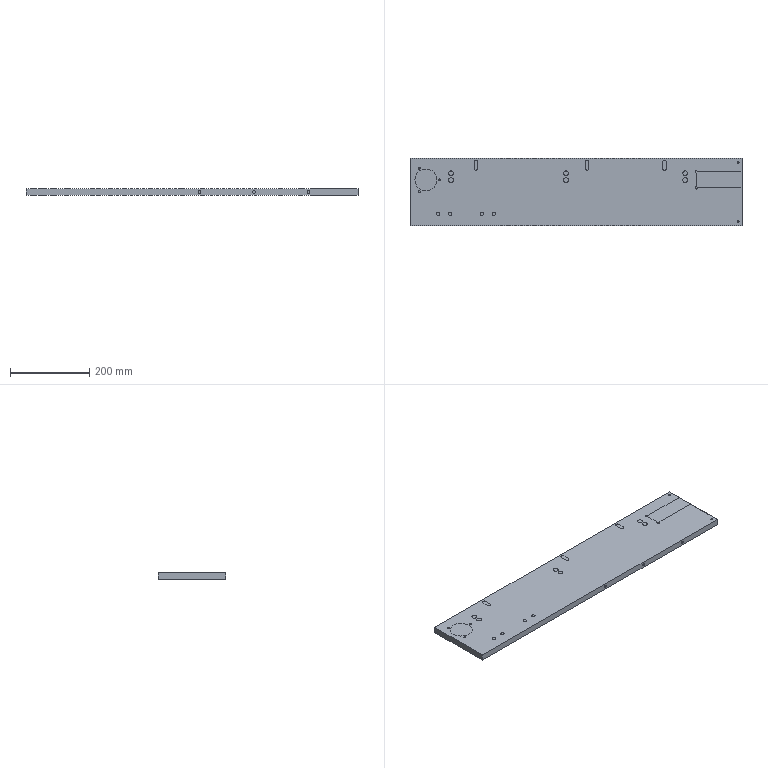NC program | NX | posted with a generic post | part box 836 x 170 x 16 mm
Lines 238 to 1148 of 11551:
(等高外形_2 , TOOL : D8平底刀)
N462 T15 M6
N464 /M1
N466 G17 G43 G0 G90 X640.643 Y150.661 Z100. S2600 H15 M3
N468 Z0.
N470 G94 G1 Z-0.2 F1200.
N472 G3 X641.5 Y152.5 R2.4
N474 G1 Y160.5 F1500.
N476 G3 X641. Y161. R0.5
N478 X640.5 Y160.5 R0.5
N480 G1 Y144.5
N482 G3 X641. Y144. R0.5
N484 X641.5 Y144.5 R0.5
N486 G1 Y152.5
N488 Y160.5 Z-0.246
N490 X641.483 Y160.628
N492 X641.463 Y160.689 Z-0.247
N494 X641.407 Y160.79
N496 X641.357 Y160.85 Z-0.248
N498 X641.269 Y160.922
N500 X641.199 Y160.959 Z-0.249
N502 X641.088 Y160.992 Z-0.25
N504 X641.006 Y161.
N506 X640.891 Y160.988 Z-0.251
N508 X640.813 Y160.964
N510 X640.712 Y160.909 Z-0.252
N512 X640.649 Y160.856
N514 X640.576 Y160.766 Z-0.253
N516 X640.539 Y160.693
N518 X640.513 Y160.615 Z-0.254
N520 X640.5 Y160.5
N522 Y144.5 Z-0.346
N524 X640.517 Y144.37
N526 X640.539 Y144.307 Z-0.347
N528 X640.597 Y144.204
N530 X640.649 Y144.144 Z-0.348
N532 X640.74 Y144.073
N534 X640.814 Y144.036 Z-0.349
N536 X640.925 Y144.006 Z-0.35
N538 X641.007 Y144.
N540 X641.121 Y144.015 Z-0.351
N542 X641.199 Y144.041
N544 X641.297 Y144.098 Z-0.352
N546 X641.358 Y144.151
N548 X641.427 Y144.24 Z-0.353
N550 X641.463 Y144.311
N552 X641.487 Y144.388 Z-0.354
N554 X641.5 Y144.5
N556 Y152.5 Z-0.4
N558 Y160.5 Z-0.446
N560 X641.483 Y160.628
N562 X641.463 Y160.689 Z-0.447
N564 X641.407 Y160.79
N566 X641.357 Y160.85 Z-0.448
N568 X641.269 Y160.922
N570 X641.199 Y160.959 Z-0.449
N572 X641.088 Y160.992 Z-0.45
N574 X641.006 Y161.
N576 X640.891 Y160.988 Z-0.451
N578 X640.813 Y160.964
N580 X640.712 Y160.909 Z-0.452
N582 X640.649 Y160.856
N584 X640.576 Y160.766 Z-0.453
N586 X640.539 Y160.693
N588 X640.513 Y160.615 Z-0.454
N590 X640.5 Y160.5
N592 Y144.5 Z-0.546
N594 X640.517 Y144.37
N596 X640.539 Y144.307 Z-0.547
N598 X640.597 Y144.204
N600 X640.649 Y144.144 Z-0.548
N602 X640.74 Y144.073
N604 X640.814 Y144.036 Z-0.549
N606 X640.925 Y144.006 Z-0.55
N608 X641.007 Y144.
N610 X641.121 Y144.015 Z-0.551
N612 X641.199 Y144.041
N614 X641.297 Y144.098 Z-0.552
N616 X641.358 Y144.151
N618 X641.427 Y144.24 Z-0.553
N620 X641.463 Y144.311
N622 X641.487 Y144.388 Z-0.554
N624 X641.5 Y144.5
N626 Y152.5 Z-0.6
N628 Y160.5 Z-0.646
N630 X641.483 Y160.628
N632 X641.463 Y160.689 Z-0.647
N634 X641.407 Y160.79
N636 X641.357 Y160.85 Z-0.648
N638 X641.269 Y160.922
N640 X641.199 Y160.959 Z-0.649
N642 X641.088 Y160.992 Z-0.65
N644 X641.006 Y161.
N646 X640.891 Y160.988 Z-0.651
N648 X640.813 Y160.964
N650 X640.712 Y160.909 Z-0.652
N652 X640.649 Y160.856
N654 X640.576 Y160.766 Z-0.653
N656 X640.539 Y160.693
N658 X640.513 Y160.615 Z-0.654
N660 X640.5 Y160.5
N662 Y144.5 Z-0.746
N664 X640.517 Y144.37
N666 X640.539 Y144.307 Z-0.747
N668 X640.597 Y144.204
N670 X640.649 Y144.144 Z-0.748
N672 X640.74 Y144.073
N674 X640.814 Y144.036 Z-0.749
N676 X640.925 Y144.006 Z-0.75
N678 X641.007 Y144.
N680 X641.121 Y144.015 Z-0.751
N682 X641.199 Y144.041
N684 X641.297 Y144.098 Z-0.752
N686 X641.358 Y144.151
N688 X641.427 Y144.24 Z-0.753
N690 X641.463 Y144.311
N692 X641.487 Y144.388 Z-0.754
N694 X641.5 Y144.5
N696 Y152.5 Z-0.8
N698 Y160.5 Z-0.846
N700 X641.483 Y160.628
N702 X641.463 Y160.689 Z-0.847
N704 X641.407 Y160.79
N706 X641.357 Y160.85 Z-0.848
N708 X641.269 Y160.922
N710 X641.199 Y160.959 Z-0.849
N712 X641.088 Y160.992 Z-0.85
N714 X641.006 Y161.
N716 X640.891 Y160.988 Z-0.851
N718 X640.813 Y160.964
N720 X640.712 Y160.909 Z-0.852
N722 X640.649 Y160.856
N724 X640.576 Y160.766 Z-0.853
N726 X640.539 Y160.693
N728 X640.513 Y160.615 Z-0.854
N730 X640.5 Y160.5
N732 Y144.5 Z-0.946
N734 X640.517 Y144.37
N736 X640.539 Y144.307 Z-0.947
N738 X640.597 Y144.204
N740 X640.649 Y144.144 Z-0.948
N742 X640.74 Y144.073
N744 X640.814 Y144.036 Z-0.949
N746 X640.925 Y144.006 Z-0.95
N748 X641.007 Y144.
N750 X641.121 Y144.015 Z-0.951
N752 X641.199 Y144.041
N754 X641.297 Y144.098 Z-0.952
N756 X641.358 Y144.151
N758 X641.427 Y144.24 Z-0.953
N760 X641.463 Y144.311
N762 X641.487 Y144.388 Z-0.954
N764 X641.5 Y144.5
N766 Y152.5 Z-1.
N768 Y160.5 Z-1.046
N770 X641.483 Y160.628
N772 X641.463 Y160.689 Z-1.047
N774 X641.407 Y160.79
N776 X641.357 Y160.85 Z-1.048
N778 X641.269 Y160.922
N780 X641.199 Y160.959 Z-1.049
N782 X641.088 Y160.992 Z-1.05
N784 X641.006 Y161.
N786 X640.891 Y160.988 Z-1.051
N788 X640.813 Y160.964
N790 X640.712 Y160.909 Z-1.052
N792 X640.649 Y160.856
N794 X640.576 Y160.766 Z-1.053
N796 X640.539 Y160.693
N798 X640.513 Y160.615 Z-1.054
N800 X640.5 Y160.5
N802 Y144.5 Z-1.146
N804 X640.517 Y144.37
N806 X640.539 Y144.307 Z-1.147
N808 X640.597 Y144.204
N810 X640.649 Y144.144 Z-1.148
N812 X640.74 Y144.073
N814 X640.814 Y144.036 Z-1.149
N816 X640.925 Y144.006 Z-1.15
N818 X641.007 Y144.
N820 X641.121 Y144.015 Z-1.151
N822 X641.199 Y144.041
N824 X641.297 Y144.098 Z-1.152
N826 X641.358 Y144.151
N828 X641.427 Y144.24 Z-1.153
N830 X641.463 Y144.311
N832 X641.487 Y144.388 Z-1.154
N834 X641.5 Y144.5
N836 Y152.5 Z-1.2
N838 Y160.5 Z-1.246
N840 X641.483 Y160.628
N842 X641.463 Y160.689 Z-1.247
N844 X641.407 Y160.79
N846 X641.357 Y160.85 Z-1.248
N848 X641.269 Y160.922
N850 X641.199 Y160.959 Z-1.249
N852 X641.088 Y160.992 Z-1.25
N854 X641.006 Y161.
N856 X640.891 Y160.988 Z-1.251
N858 X640.813 Y160.964
N860 X640.712 Y160.909 Z-1.252
N862 X640.649 Y160.856
N864 X640.576 Y160.766 Z-1.253
N866 X640.539 Y160.693
N868 X640.513 Y160.615 Z-1.254
N870 X640.5 Y160.5
N872 Y144.5 Z-1.346
N874 X640.517 Y144.37
N876 X640.539 Y144.307 Z-1.347
N878 X640.597 Y144.204
N880 X640.649 Y144.144 Z-1.348
N882 X640.74 Y144.073
N884 X640.814 Y144.036 Z-1.349
N886 X640.925 Y144.006 Z-1.35
N888 X641.007 Y144.
N890 X641.121 Y144.015 Z-1.351
N892 X641.199 Y144.041
N894 X641.297 Y144.098 Z-1.352
N896 X641.358 Y144.151
N898 X641.427 Y144.24 Z-1.353
N900 X641.463 Y144.311
N902 X641.487 Y144.388 Z-1.354
N904 X641.5 Y144.5
N906 Y152.5 Z-1.4
N908 Y160.5 Z-1.446
N910 X641.483 Y160.628
N912 X641.463 Y160.689 Z-1.447
N914 X641.407 Y160.79
N916 X641.357 Y160.85 Z-1.448
N918 X641.269 Y160.922
N920 X641.199 Y160.959 Z-1.449
N922 X641.088 Y160.992 Z-1.45
N924 X641.006 Y161.
N926 X640.891 Y160.988 Z-1.451
N928 X640.813 Y160.964
N930 X640.712 Y160.909 Z-1.452
N932 X640.649 Y160.856
N934 X640.576 Y160.766 Z-1.453
N936 X640.539 Y160.693
N938 X640.513 Y160.615 Z-1.454
N940 X640.5 Y160.5
N942 Y144.5 Z-1.546
N944 X640.517 Y144.37
N946 X640.539 Y144.307 Z-1.547
N948 X640.597 Y144.204
N950 X640.649 Y144.144 Z-1.548
N952 X640.74 Y144.073
N954 X640.814 Y144.036 Z-1.549
N956 X640.925 Y144.006 Z-1.55
N958 X641.007 Y144.
N960 X641.121 Y144.015 Z-1.551
N962 X641.199 Y144.041
N964 X641.297 Y144.098 Z-1.552
N966 X641.358 Y144.151
N968 X641.427 Y144.24 Z-1.553
N970 X641.463 Y144.311
N972 X641.487 Y144.388 Z-1.554
N974 X641.5 Y144.5
N976 Y152.5 Z-1.6
N978 Y160.5 Z-1.646
N980 X641.483 Y160.628
N982 X641.463 Y160.689 Z-1.647
N984 X641.407 Y160.79
N986 X641.357 Y160.85 Z-1.648
N988 X641.269 Y160.922
N990 X641.199 Y160.959 Z-1.649
N992 X641.088 Y160.992 Z-1.65
N994 X641.006 Y161.
N996 X640.891 Y160.988 Z-1.651
N998 X640.813 Y160.964
N1000 X640.712 Y160.909 Z-1.652
N1002 X640.649 Y160.856
N1004 X640.576 Y160.766 Z-1.653
N1006 X640.539 Y160.693
N1008 X640.513 Y160.615 Z-1.654
N1010 X640.5 Y160.5
N1012 Y144.5 Z-1.746
N1014 X640.517 Y144.37
N1016 X640.539 Y144.307 Z-1.747
N1018 X640.597 Y144.204
N1020 X640.649 Y144.144 Z-1.748
N1022 X640.74 Y144.073
N1024 X640.814 Y144.036 Z-1.749
N1026 X640.925 Y144.006 Z-1.75
N1028 X641.007 Y144.
N1030 X641.121 Y144.015 Z-1.751
N1032 X641.199 Y144.041
N1034 X641.297 Y144.098 Z-1.752
N1036 X641.358 Y144.151
N1038 X641.427 Y144.24 Z-1.753
N1040 X641.463 Y144.311
N1042 X641.487 Y144.388 Z-1.754
N1044 X641.5 Y144.5
N1046 Y152.5 Z-1.8
N1048 Y160.5 Z-1.846
N1050 X641.483 Y160.628
N1052 X641.463 Y160.689 Z-1.847
N1054 X641.407 Y160.79
N1056 X641.357 Y160.85 Z-1.848
N1058 X641.269 Y160.922
N1060 X641.199 Y160.959 Z-1.849
N1062 X641.088 Y160.992 Z-1.85
N1064 X641.006 Y161.
N1066 X640.891 Y160.988 Z-1.851
N1068 X640.813 Y160.964
N1070 X640.712 Y160.909 Z-1.852
N1072 X640.649 Y160.856
N1074 X640.576 Y160.766 Z-1.853
N1076 X640.539 Y160.693
N1078 X640.513 Y160.615 Z-1.854
N1080 X640.5 Y160.5
N1082 Y144.5 Z-1.946
N1084 X640.517 Y144.37
N1086 X640.539 Y144.307 Z-1.947
N1088 X640.597 Y144.204
N1090 X640.649 Y144.144 Z-1.948
N1092 X640.74 Y144.073
N1094 X640.814 Y144.036 Z-1.949
N1096 X640.925 Y144.006 Z-1.95
N1098 X641.007 Y144.
N1100 X641.121 Y144.015 Z-1.951
N1102 X641.199 Y144.041
N1104 X641.297 Y144.098 Z-1.952
N1106 X641.358 Y144.151
N1108 X641.427 Y144.24 Z-1.953
N1110 X641.463 Y144.311
N1112 X641.487 Y144.388 Z-1.954
N1114 X641.5 Y144.5
N1116 Y152.5 Z-2.
N1118 Y160.5 Z-2.046
N1120 X641.483 Y160.628
N1122 X641.463 Y160.689 Z-2.047
N1124 X641.407 Y160.79
N1126 X641.357 Y160.85 Z-2.048
N1128 X641.269 Y160.922
N1130 X641.199 Y160.959 Z-2.049
N1132 X641.088 Y160.992 Z-2.05
N1134 X641.006 Y161.
N1136 X640.891 Y160.988 Z-2.051
N1138 X640.813 Y160.964
N1140 X640.712 Y160.909 Z-2.052
N1142 X640.649 Y160.856
N1144 X640.576 Y160.766 Z-2.053
N1146 X640.539 Y160.693
N1148 X640.513 Y160.615 Z-2.054
N1150 X640.5 Y160.5
N1152 Y144.5 Z-2.146
N1154 X640.517 Y144.37
N1156 X640.539 Y144.307 Z-2.147
N1158 X640.597 Y144.204
N1160 X640.649 Y144.144 Z-2.148
N1162 X640.74 Y144.073
N1164 X640.814 Y144.036 Z-2.149
N1166 X640.925 Y144.006 Z-2.15
N1168 X641.007 Y144.
N1170 X641.121 Y144.015 Z-2.151
N1172 X641.199 Y144.041
N1174 X641.297 Y144.098 Z-2.152
N1176 X641.358 Y144.151
N1178 X641.427 Y144.24 Z-2.153
N1180 X641.463 Y144.311
N1182 X641.487 Y144.388 Z-2.154
N1184 X641.5 Y144.5
N1186 Y152.5 Z-2.2
N1188 Y160.5 Z-2.246
N1190 X641.483 Y160.628
N1192 X641.463 Y160.689 Z-2.247
N1194 X641.407 Y160.79
N1196 X641.357 Y160.85 Z-2.248
N1198 X641.269 Y160.922
N1200 X641.199 Y160.959 Z-2.249
N1202 X641.088 Y160.992 Z-2.25
N1204 X641.006 Y161.
N1206 X640.891 Y160.988 Z-2.251
N1208 X640.813 Y160.964
N1210 X640.712 Y160.909 Z-2.252
N1212 X640.649 Y160.856
N1214 X640.576 Y160.766 Z-2.253
N1216 X640.539 Y160.693
N1218 X640.513 Y160.615 Z-2.254
N1220 X640.5 Y160.5
N1222 Y144.5 Z-2.346
N1224 X640.517 Y144.37
N1226 X640.539 Y144.307 Z-2.347
N1228 X640.597 Y144.204
N1230 X640.649 Y144.144 Z-2.348
N1232 X640.74 Y144.073
N1234 X640.814 Y144.036 Z-2.349
N1236 X640.925 Y144.006 Z-2.35
N1238 X641.007 Y144.
N1240 X641.121 Y144.015 Z-2.351
N1242 X641.199 Y144.041
N1244 X641.297 Y144.098 Z-2.352
N1246 X641.358 Y144.151
N1248 X641.427 Y144.24 Z-2.353
N1250 X641.463 Y144.311
N1252 X641.487 Y144.388 Z-2.354
N1254 X641.5 Y144.5
N1256 Y152.5 Z-2.4
N1258 Y160.5 Z-2.446
N1260 X641.483 Y160.628
N1262 X641.463 Y160.689 Z-2.447
N1264 X641.407 Y160.79
N1266 X641.357 Y160.85 Z-2.448
N1268 X641.269 Y160.922
N1270 X641.199 Y160.959 Z-2.449
N1272 X641.088 Y160.992 Z-2.45
N1274 X641.006 Y161.
N1276 X640.891 Y160.988 Z-2.451
N1278 X640.813 Y160.964
N1280 X640.712 Y160.909 Z-2.452
N1282 X640.649 Y160.856
N1284 X640.576 Y160.766 Z-2.453
N1286 X640.539 Y160.693
N1288 X640.513 Y160.615 Z-2.454
N1290 X640.5 Y160.5
N1292 Y144.5 Z-2.546
N1294 X640.517 Y144.37
N1296 X640.539 Y144.307 Z-2.547
N1298 X640.597 Y144.204
N1300 X640.649 Y144.144 Z-2.548
N1302 X640.74 Y144.073
N1304 X640.814 Y144.036 Z-2.549
N1306 X640.925 Y144.006 Z-2.55
N1308 X641.007 Y144.
N1310 X641.121 Y144.015 Z-2.551
N1312 X641.199 Y144.041
N1314 X641.297 Y144.098 Z-2.552
N1316 X641.358 Y144.151
N1318 X641.427 Y144.24 Z-2.553
N1320 X641.463 Y144.311
N1322 X641.487 Y144.388 Z-2.554
N1324 X641.5 Y144.5
N1326 Y152.5 Z-2.6
N1328 Y160.5 Z-2.646
N1330 X641.483 Y160.628
N1332 X641.463 Y160.689 Z-2.647
N1334 X641.407 Y160.79
N1336 X641.357 Y160.85 Z-2.648
N1338 X641.269 Y160.922
N1340 X641.199 Y160.959 Z-2.649
N1342 X641.088 Y160.992 Z-2.65
N1344 X641.006 Y161.
N1346 X640.891 Y160.988 Z-2.651
N1348 X640.813 Y160.964
N1350 X640.712 Y160.909 Z-2.652
N1352 X640.649 Y160.856
N1354 X640.576 Y160.766 Z-2.653
N1356 X640.539 Y160.693
N1358 X640.513 Y160.615 Z-2.654
N1360 X640.5 Y160.5
N1362 Y144.5 Z-2.746
N1364 X640.517 Y144.37
N1366 X640.539 Y144.307 Z-2.747
N1368 X640.597 Y144.204
N1370 X640.649 Y144.144 Z-2.748
N1372 X640.74 Y144.073
N1374 X640.814 Y144.036 Z-2.749
N1376 X640.925 Y144.006 Z-2.75
N1378 X641.007 Y144.
N1380 X641.121 Y144.015 Z-2.751
N1382 X641.199 Y144.041
N1384 X641.297 Y144.098 Z-2.752
N1386 X641.358 Y144.151
N1388 X641.427 Y144.24 Z-2.753
N1390 X641.463 Y144.311
N1392 X641.487 Y144.388 Z-2.754
N1394 X641.5 Y144.5
N1396 Y152.5 Z-2.8
N1398 Y160.5 Z-2.846
N1400 X641.483 Y160.628
N1402 X641.463 Y160.689 Z-2.847
N1404 X641.407 Y160.79
N1406 X641.357 Y160.85 Z-2.848
N1408 X641.269 Y160.922
N1410 X641.199 Y160.959 Z-2.849
N1412 X641.088 Y160.992 Z-2.85
N1414 X641.006 Y161.
N1416 X640.891 Y160.988 Z-2.851
N1418 X640.813 Y160.964
N1420 X640.712 Y160.909 Z-2.852
N1422 X640.649 Y160.856
N1424 X640.576 Y160.766 Z-2.853
N1426 X640.539 Y160.693
N1428 X640.513 Y160.615 Z-2.854
N1430 X640.5 Y160.5
N1432 Y144.5 Z-2.946
N1434 X640.517 Y144.37
N1436 X640.539 Y144.307 Z-2.947
N1438 X640.597 Y144.204
N1440 X640.649 Y144.144 Z-2.948
N1442 X640.74 Y144.073
N1444 X640.814 Y144.036 Z-2.949
N1446 X640.925 Y144.006 Z-2.95
N1448 X641.007 Y144.
N1450 X641.121 Y144.015 Z-2.951
N1452 X641.199 Y144.041
N1454 X641.297 Y144.098 Z-2.952
N1456 X641.358 Y144.151
N1458 X641.427 Y144.24 Z-2.953
N1460 X641.463 Y144.311
N1462 X641.487 Y144.388 Z-2.954
N1464 X641.5 Y144.5
N1466 Y152.5 Z-3.
N1468 Y160.5 Z-3.046
N1470 X641.483 Y160.628
N1472 X641.463 Y160.689 Z-3.047
N1474 X641.407 Y160.79
N1476 X641.357 Y160.85 Z-3.048
N1478 X641.269 Y160.922
N1480 X641.199 Y160.959 Z-3.049
N1482 X641.088 Y160.992 Z-3.05
N1484 X641.006 Y161.
N1486 X640.891 Y160.988 Z-3.051
N1488 X640.813 Y160.964
N1490 X640.712 Y160.909 Z-3.052
N1492 X640.649 Y160.856
N1494 X640.576 Y160.766 Z-3.053
N1496 X640.539 Y160.693
N1498 X640.513 Y160.615 Z-3.054
N1500 X640.5 Y160.5
N1502 Y144.5 Z-3.146
N1504 X640.517 Y144.37
N1506 X640.539 Y144.307 Z-3.147
N1508 X640.597 Y144.204
N1510 X640.649 Y144.144 Z-3.148
N1512 X640.74 Y144.073
N1514 X640.814 Y144.036 Z-3.149
N1516 X640.925 Y144.006 Z-3.15
N1518 X641.007 Y144.
N1520 X641.121 Y144.015 Z-3.151
N1522 X641.199 Y144.041
N1524 X641.297 Y144.098 Z-3.152
N1526 X641.358 Y144.151
N1528 X641.427 Y144.24 Z-3.153
N1530 X641.463 Y144.311
N1532 X641.487 Y144.388 Z-3.154
N1534 X641.5 Y144.5
N1536 Y152.5 Z-3.2
N1538 Y160.5 Z-3.246
N1540 X641.483 Y160.628
N1542 X641.463 Y160.689 Z-3.247
N1544 X641.407 Y160.79
N1546 X641.357 Y160.85 Z-3.248
N1548 X641.269 Y160.922
N1550 X641.199 Y160.959 Z-3.249
N1552 X641.088 Y160.992 Z-3.25
N1554 X641.006 Y161.
N1556 X640.891 Y160.988 Z-3.251
N1558 X640.813 Y160.964
N1560 X640.712 Y160.909 Z-3.252
N1562 X640.649 Y160.856
N1564 X640.576 Y160.766 Z-3.253
N1566 X640.539 Y160.693
N1568 X640.513 Y160.615 Z-3.254
N1570 X640.5 Y160.5
N1572 Y144.5 Z-3.346
N1574 X640.517 Y144.37
N1576 X640.539 Y144.307 Z-3.347
N1578 X640.597 Y144.204
N1580 X640.649 Y144.144 Z-3.348
N1582 X640.74 Y144.073
N1584 X640.814 Y144.036 Z-3.349
N1586 X640.925 Y144.006 Z-3.35
N1588 X641.007 Y144.
N1590 X641.121 Y144.015 Z-3.351
N1592 X641.199 Y144.041
N1594 X641.297 Y144.098 Z-3.352
N1596 X641.358 Y144.151
N1598 X641.427 Y144.24 Z-3.353
N1600 X641.463 Y144.311
N1602 X641.487 Y144.388 Z-3.354
N1604 X641.5 Y144.5
N1606 Y152.5 Z-3.4
N1608 Y160.5 Z-3.446
N1610 X641.483 Y160.628
N1612 X641.463 Y160.689 Z-3.447
N1614 X641.407 Y160.79
N1616 X641.357 Y160.85 Z-3.448
N1618 X641.269 Y160.922
N1620 X641.199 Y160.959 Z-3.449
N1622 X641.088 Y160.992 Z-3.45
N1624 X641.006 Y161.
N1626 X640.891 Y160.988 Z-3.451
N1628 X640.813 Y160.964
N1630 X640.712 Y160.909 Z-3.452
N1632 X640.649 Y160.856
N1634 X640.576 Y160.766 Z-3.453
N1636 X640.539 Y160.693
N1638 X640.513 Y160.615 Z-3.454
N1640 X640.5 Y160.5
N1642 Y144.5 Z-3.546
N1644 X640.517 Y144.37
N1646 X640.539 Y144.307 Z-3.547
N1648 X640.597 Y144.204
N1650 X640.649 Y144.144 Z-3.548
N1652 X640.74 Y144.073
N1654 X640.814 Y144.036 Z-3.549
N1656 X640.925 Y144.006 Z-3.55
N1658 X641.007 Y144.
N1660 X641.121 Y144.015 Z-3.551
N1662 X641.199 Y144.041
N1664 X641.297 Y144.098 Z-3.552
N1666 X641.358 Y144.151
N1668 X641.427 Y144.24 Z-3.553
N1670 X641.463 Y144.311
N1672 X641.487 Y144.388 Z-3.554
N1674 X641.5 Y144.5
N1676 Y152.5 Z-3.6
N1678 Y160.5 Z-3.646
N1680 X641.483 Y160.628
N1682 X641.463 Y160.689 Z-3.647
N1684 X641.407 Y160.79
N1686 X641.357 Y160.85 Z-3.648
N1688 X641.269 Y160.922
N1690 X641.199 Y160.959 Z-3.649
N1692 X641.088 Y160.992 Z-3.65
N1694 X641.006 Y161.
N1696 X640.891 Y160.988 Z-3.651
N1698 X640.813 Y160.964
N1700 X640.712 Y160.909 Z-3.652
N1702 X640.649 Y160.856
N1704 X640.576 Y160.766 Z-3.653
N1706 X640.539 Y160.693
N1708 X640.513 Y160.615 Z-3.654
N1710 X640.5 Y160.5
N1712 Y144.5 Z-3.746
N1714 X640.517 Y144.37
N1716 X640.539 Y144.307 Z-3.747
N1718 X640.597 Y144.204
N1720 X640.649 Y144.144 Z-3.748
N1722 X640.74 Y144.073
N1724 X640.814 Y144.036 Z-3.749
N1726 X640.925 Y144.006 Z-3.75
N1728 X641.007 Y144.
N1730 X641.121 Y144.015 Z-3.751
N1732 X641.199 Y144.041
N1734 X641.297 Y144.098 Z-3.752
N1736 X641.358 Y144.151
N1738 X641.427 Y144.24 Z-3.753
N1740 X641.463 Y144.311
N1742 X641.487 Y144.388 Z-3.754
N1744 X641.5 Y144.5
N1746 Y152.5 Z-3.8
N1748 Y160.5 Z-3.846
N1750 X641.483 Y160.628
N1752 X641.463 Y160.689 Z-3.847
N1754 X641.407 Y160.79
N1756 X641.357 Y160.85 Z-3.848
N1758 X641.269 Y160.922
N1760 X641.199 Y160.959 Z-3.849
N1762 X641.088 Y160.992 Z-3.85
N1764 X641.006 Y161.
N1766 X640.891 Y160.988 Z-3.851
N1768 X640.813 Y160.964
N1770 X640.712 Y160.909 Z-3.852
N1772 X640.649 Y160.856
N1774 X640.576 Y160.766 Z-3.853
N1776 X640.539 Y160.693
N1778 X640.513 Y160.615 Z-3.854
N1780 X640.5 Y160.5
N1782 Y144.5 Z-3.946
N1784 X640.517 Y144.37
N1786 X640.539 Y144.307 Z-3.947
N1788 X640.597 Y144.204
N1790 X640.649 Y144.144 Z-3.948
N1792 X640.74 Y144.073
N1794 X640.814 Y144.036 Z-3.949
N1796 X640.925 Y144.006 Z-3.95
N1798 X641.007 Y144.
N1800 X641.121 Y144.015 Z-3.951
N1802 X641.199 Y144.041
N1804 X641.297 Y144.098 Z-3.952
N1806 X641.358 Y144.151
N1808 X641.427 Y144.24 Z-3.953
N1810 X641.463 Y144.311
N1812 X641.487 Y144.388 Z-3.954
N1814 X641.5 Y144.5
N1816 Y152.5 Z-4.
N1818 Y160.5 Z-4.046
N1820 X641.483 Y160.628
N1822 X641.463 Y160.689 Z-4.047
N1824 X641.407 Y160.79
N1826 X641.357 Y160.85 Z-4.048
N1828 X641.269 Y160.922
N1830 X641.199 Y160.959 Z-4.049
N1832 X641.088 Y160.992 Z-4.05
N1834 X641.006 Y161.
N1836 X640.891 Y160.988 Z-4.051
N1838 X640.813 Y160.964
N1840 X640.712 Y160.909 Z-4.052
N1842 X640.649 Y160.856
N1844 X640.576 Y160.766 Z-4.053
N1846 X640.539 Y160.693
N1848 X640.513 Y160.615 Z-4.054
N1850 X640.5 Y160.5
N1852 Y144.5 Z-4.146
N1854 X640.517 Y144.37
N1856 X640.539 Y144.307 Z-4.147
N1858 X640.597 Y144.204
N1860 X640.649 Y144.144 Z-4.148
N1862 X640.74 Y144.073
N1864 X640.814 Y144.036 Z-4.149
N1866 X640.925 Y144.006 Z-4.15
N1868 X641.007 Y144.
N1870 X641.121 Y144.015 Z-4.151
N1872 X641.199 Y144.041
N1874 X641.297 Y144.098 Z-4.152
N1876 X641.358 Y144.151
N1878 X641.427 Y144.24 Z-4.153
N1880 X641.463 Y144.311
N1882 X641.487 Y144.388 Z-4.154
N1884 X641.5 Y144.5
N1886 Y152.5 Z-4.2
N1888 Y160.5 Z-4.246
N1890 X641.483 Y160.628
N1892 X641.463 Y160.689 Z-4.247
N1894 X641.407 Y160.79
N1896 X641.357 Y160.85 Z-4.248
N1898 X641.269 Y160.922
N1900 X641.199 Y160.959 Z-4.249
N1902 X641.088 Y160.992 Z-4.25
N1904 X641.006 Y161.
N1906 X640.891 Y160.988 Z-4.251
N1908 X640.813 Y160.964
N1910 X640.712 Y160.909 Z-4.252
N1912 X640.649 Y160.856
N1914 X640.576 Y160.766 Z-4.253
N1916 X640.539 Y160.693
N1918 X640.513 Y160.615 Z-4.254
N1920 X640.5 Y160.5
N1922 Y144.5 Z-4.346
N1924 X640.517 Y144.37
N1926 X640.539 Y144.307 Z-4.347
N1928 X640.597 Y144.204
N1930 X640.649 Y144.144 Z-4.348
N1932 X640.74 Y144.073
N1934 X640.814 Y144.036 Z-4.349
N1936 X640.925 Y144.006 Z-4.35
N1938 X641.007 Y144.
N1940 X641.121 Y144.015 Z-4.351
N1942 X641.199 Y144.041
N1944 X641.297 Y144.098 Z-4.352
N1946 X641.358 Y144.151
N1948 X641.427 Y144.24 Z-4.353
N1950 X641.463 Y144.311
N1952 X641.487 Y144.388 Z-4.354
N1954 X641.5 Y144.5
N1956 Y152.5 Z-4.4
N1958 Y160.5 Z-4.446
N1960 X641.483 Y160.628
N1962 X641.463 Y160.689 Z-4.447
N1964 X641.407 Y160.79
N1966 X641.357 Y160.85 Z-4.448
N1968 X641.269 Y160.922
N1970 X641.199 Y160.959 Z-4.449
N1972 X641.088 Y160.992 Z-4.45
N1974 X641.006 Y161.
N1976 X640.891 Y160.988 Z-4.451
N1978 X640.813 Y160.964
N1980 X640.712 Y160.909 Z-4.452
N1982 X640.649 Y160.856
N1984 X640.576 Y160.766 Z-4.453
N1986 X640.539 Y160.693
N1988 X640.513 Y160.615 Z-4.454
N1990 X640.5 Y160.5
N1992 Y144.5 Z-4.546
N1994 X640.517 Y144.37
N1996 X640.539 Y144.307 Z-4.547
N1998 X640.597 Y144.204
N2000 X640.649 Y144.144 Z-4.548
N2002 X640.74 Y144.073
N2004 X640.814 Y144.036 Z-4.549
N2006 X640.925 Y144.006 Z-4.55
N2008 X641.007 Y144.
N2010 X641.121 Y144.015 Z-4.551
N2012 X641.199 Y144.041
N2014 X641.297 Y144.098 Z-4.552
N2016 X641.358 Y144.151
N2018 X641.427 Y144.24 Z-4.553
N2020 X641.463 Y144.311
N2022 X641.487 Y144.388 Z-4.554
N2024 X641.5 Y144.5
N2026 Y152.5 Z-4.6
N2028 Y160.5 Z-4.646
N2030 X641.483 Y160.628
N2032 X641.463 Y160.689 Z-4.647
N2034 X641.407 Y160.79
N2036 X641.357 Y160.85 Z-4.648
N2038 X641.269 Y160.922
N2040 X641.199 Y160.959 Z-4.649
N2042 X641.088 Y160.992 Z-4.65
N2044 X641.006 Y161.
N2046 X640.891 Y160.988 Z-4.651
N2048 X640.813 Y160.964
N2050 X640.712 Y160.909 Z-4.652
N2052 X640.649 Y160.856
N2054 X640.576 Y160.766 Z-4.653
N2056 X640.539 Y160.693
N2058 X640.513 Y160.615 Z-4.654
N2060 X640.5 Y160.5
N2062 Y144.5 Z-4.746
N2064 X640.517 Y144.37
N2066 X640.539 Y144.307 Z-4.747
N2068 X640.597 Y144.204
N2070 X640.649 Y144.144 Z-4.748
N2072 X640.74 Y144.073
N2074 X640.814 Y144.036 Z-4.749
N2076 X640.925 Y144.006 Z-4.75
N2078 X641.007 Y144.
N2080 X641.121 Y144.015 Z-4.751
N2082 X641.199 Y144.041
N2084 X641.297 Y144.098 Z-4.752
N2086 X641.358 Y144.151
N2088 X641.427 Y144.24 Z-4.753
N2090 X641.463 Y144.311
N2092 X641.487 Y144.388 Z-4.754
N2094 X641.5 Y144.5
N2096 Y152.5 Z-4.8
N2098 Y160.5 Z-4.846
N2100 X641.483 Y160.628
N2102 X641.463 Y160.689 Z-4.847
N2104 X641.407 Y160.79
N2106 X641.357 Y160.85 Z-4.848
N2108 X641.269 Y160.922
N2110 X641.199 Y160.959 Z-4.849
N2112 X641.088 Y160.992 Z-4.85
N2114 X641.006 Y161.
N2116 X640.891 Y160.988 Z-4.851
N2118 X640.813 Y160.964
N2120 X640.712 Y160.909 Z-4.852
N2122 X640.649 Y160.856
N2124 X640.576 Y160.766 Z-4.853
N2126 X640.539 Y160.693
N2128 X640.513 Y160.615 Z-4.854
N2130 X640.5 Y160.5
N2132 Y144.5 Z-4.946
N2134 X640.517 Y144.37
N2136 X640.539 Y144.307 Z-4.947
N2138 X640.597 Y144.204
N2140 X640.649 Y144.144 Z-4.948
N2142 X640.74 Y144.073
N2144 X640.814 Y144.036 Z-4.949
N2146 X640.925 Y144.006 Z-4.95
N2148 X641.007 Y144.
N2150 X641.121 Y144.015 Z-4.951
N2152 X641.199 Y144.041
N2154 X641.297 Y144.098 Z-4.952
N2156 X641.358 Y144.151
N2158 X641.427 Y144.24 Z-4.953
N2160 X641.463 Y144.311
N2162 X641.487 Y144.388 Z-4.954
N2164 X641.5 Y144.5
N2166 Y152.5 Z-5.
N2168 Y160.5 Z-5.046
N2170 X641.483 Y160.628
N2172 X641.463 Y160.689 Z-5.047
N2174 X641.407 Y160.79
N2176 X641.357 Y160.85 Z-5.048
N2178 X641.269 Y160.922
N2180 X641.199 Y160.959 Z-5.049
N2182 X641.088 Y160.992 Z-5.05
N2184 X641.006 Y161.
N2186 X640.891 Y160.988 Z-5.051
N2188 X640.813 Y160.964
N2190 X640.712 Y160.909 Z-5.052
N2192 X640.649 Y160.856
N2194 X640.576 Y160.766 Z-5.053
N2196 X640.539 Y160.693
N2198 X640.513 Y160.615 Z-5.054
N2200 X640.5 Y160.5
N2202 Y144.5 Z-5.146
N2204 X640.517 Y144.37
N2206 X640.539 Y144.307 Z-5.147
N2208 X640.597 Y144.204
N2210 X640.649 Y144.144 Z-5.148
N2212 X640.74 Y144.073
N2214 X640.814 Y144.036 Z-5.149
N2216 X640.925 Y144.006 Z-5.15
N2218 X641.007 Y144.
N2220 X641.121 Y144.015 Z-5.151
N2222 X641.199 Y144.041
N2224 X641.297 Y144.098 Z-5.152
N2226 X641.358 Y144.151
N2228 X641.427 Y144.24 Z-5.153
N2230 X641.463 Y144.311
N2232 X641.487 Y144.388 Z-5.154
N2234 X641.5 Y144.5
N2236 Y152.5 Z-5.2
N2238 Y160.5 Z-5.246
N2240 X641.483 Y160.628
N2242 X641.463 Y160.689 Z-5.247
N2244 X641.407 Y160.79
N2246 X641.357 Y160.85 Z-5.248
N2248 X641.269 Y160.922
N2250 X641.199 Y160.959 Z-5.249
N2252 X641.088 Y160.992 Z-5.25
N2254 X641.006 Y161.
N2256 X640.891 Y160.988 Z-5.251
N2258 X640.813 Y160.964
N2260 X640.712 Y160.909 Z-5.252
N2262 X640.649 Y160.856
N2264 X640.576 Y160.766 Z-5.253
N2266 X640.539 Y160.693
N2268 X640.513 Y160.615 Z-5.254
N2270 X640.5 Y160.5
N2272 Y144.5 Z-5.346
N2274 X640.517 Y144.37
N2276 X640.539 Y144.307 Z-5.347